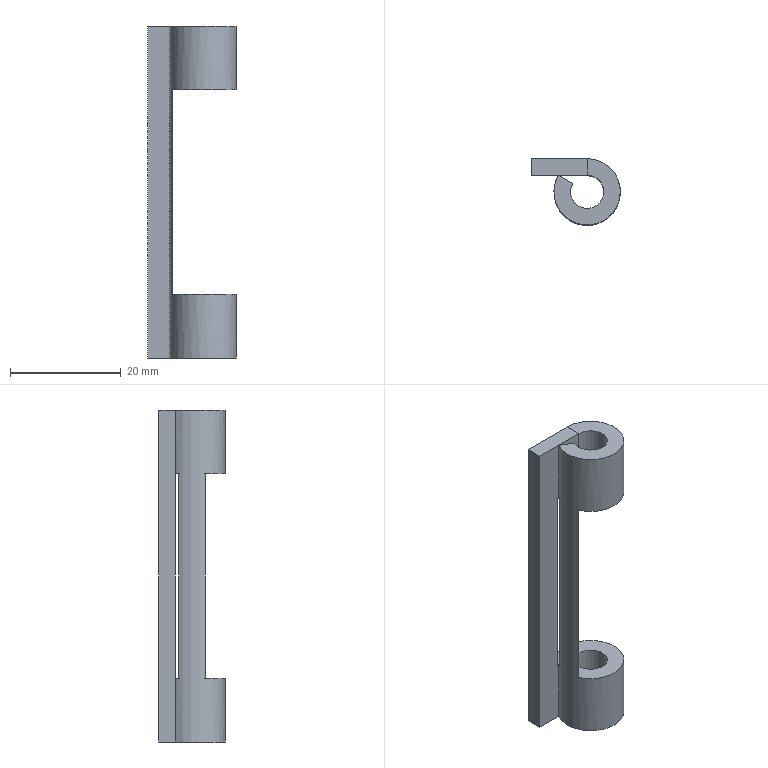Part | SolidWorks | features Cut 1, FlatPattern 1, Hem 1, SMBaseFlange 1, SheetMetal 1 | 1 solid | 16 faces | box 16 x 12 x 60 mm | volume 2875 mm3 | plane 13 | cylinder 3 | commonest cylinder face diameters 6 x2 12 x1
STEP:
#1=CARTESIAN_POINT('',(-3.5,-3.,-18.5));
#2=VERTEX_POINT('',#1);
#3=CARTESIAN_POINT('',(2.,-3.,-18.5));
#4=VERTEX_POINT('',#3);
#5=CARTESIAN_POINT('',(0.,-3.,-18.5));
#6=DIRECTION('',(1.,0.,0.));
#7=VECTOR('',#6,1000.);
#8=LINE('',#5,#7);
#9=EDGE_CURVE('',#2,#4,#8,.T.);
#10=ORIENTED_EDGE('',*,*,#9,.F.);
#11=CARTESIAN_POINT('',(-3.5,-3.,18.5));
#12=VERTEX_POINT('',#11);
#13=CARTESIAN_POINT('',(-3.5,-3.,0.));
#14=DIRECTION('',(0.,0.,1.));
#15=VECTOR('',#14,1000.);
#16=LINE('',#13,#15);
#17=EDGE_CURVE('',#2,#12,#16,.T.);
#18=ORIENTED_EDGE('',*,*,#17,.T.);
#19=CARTESIAN_POINT('',(2.,-3.,18.5));
#20=VERTEX_POINT('',#19);
#21=CARTESIAN_POINT('',(0.,-3.,18.5));
#22=DIRECTION('',(1.,0.,0.));
#23=VECTOR('',#22,1000.);
#24=LINE('',#21,#23);
#25=EDGE_CURVE('',#12,#20,#24,.T.);
#26=ORIENTED_EDGE('',*,*,#25,.T.);
#27=CARTESIAN_POINT('',(2.,-3.,30.));
#28=VERTEX_POINT('',#27);
#29=CARTESIAN_POINT('',(2.,-3.,30.));
#30=DIRECTION('',(0.,0.,-1.));
#31=VECTOR('',#30,1000.);
#32=LINE('',#29,#31);
#33=EDGE_CURVE('',#28,#20,#32,.T.);
#34=ORIENTED_EDGE('',*,*,#33,.F.);
#35=CARTESIAN_POINT('',(-8.,-3.,30.));
#36=VERTEX_POINT('',#35);
#37=CARTESIAN_POINT('',(-8.,-3.,30.));
#38=DIRECTION('',(1.,0.,0.));
#39=VECTOR('',#38,1000.);
#40=LINE('',#37,#39);
#41=EDGE_CURVE('',#36,#28,#40,.T.);
#42=ORIENTED_EDGE('',*,*,#41,.F.);
#43=CARTESIAN_POINT('',(-8.,-3.,-30.));
#44=VERTEX_POINT('',#43);
#45=CARTESIAN_POINT('',(-8.,-3.,-30.));
#46=DIRECTION('',(0.,0.,1.));
#47=VECTOR('',#46,1000.);
#48=LINE('',#45,#47);
#49=EDGE_CURVE('',#44,#36,#48,.T.);
#50=ORIENTED_EDGE('',*,*,#49,.F.);
#51=CARTESIAN_POINT('',(2.,-3.,-30.));
#52=VERTEX_POINT('',#51);
#53=CARTESIAN_POINT('',(-8.,-3.,-30.));
#54=DIRECTION('',(-1.,0.,0.));
#55=VECTOR('',#54,1000.);
#56=LINE('',#53,#55);
#57=EDGE_CURVE('',#52,#44,#56,.T.);
#58=ORIENTED_EDGE('',*,*,#57,.F.);
#59=CARTESIAN_POINT('',(2.,-3.,30.));
#60=DIRECTION('',(0.,0.,-1.));
#61=VECTOR('',#60,1000.);
#62=LINE('',#59,#61);
#63=EDGE_CURVE('',#4,#52,#62,.T.);
#64=ORIENTED_EDGE('',*,*,#63,.F.);
#65=EDGE_LOOP('',(#10,#18,#26,#34,#42,#50,#58,#64));
#66=FACE_OUTER_BOUND('',#65,.T.);
#67=CARTESIAN_POINT('',(0.,-3.,0.));
#68=DIRECTION('',(0.,1.,0.));
#69=DIRECTION('',(0.,0.,1.));
#70=AXIS2_PLACEMENT_3D('',#67,#68,#69);
#71=PLANE('',#70);
#72=ADVANCED_FACE('',(#66),#71,.F.);
#73=CARTESIAN_POINT('',(-3.5,0.,-18.5));
#74=VERTEX_POINT('',#73);
#75=CARTESIAN_POINT('',(-3.5,0.,18.5));
#76=VERTEX_POINT('',#75);
#77=CARTESIAN_POINT('',(-3.5,0.,-18.5));
#78=DIRECTION('',(0.,0.,1.));
#79=VECTOR('',#78,1000.);
#80=LINE('',#77,#79);
#81=EDGE_CURVE('',#74,#76,#80,.T.);
#82=ORIENTED_EDGE('',*,*,#81,.F.);
#83=CARTESIAN_POINT('',(2.,0.,-18.5));
#84=VERTEX_POINT('',#83);
#85=CARTESIAN_POINT('',(-3.5,0.,-18.5));
#86=DIRECTION('',(1.,0.,0.));
#87=VECTOR('',#86,1000.);
#88=LINE('',#85,#87);
#89=EDGE_CURVE('',#74,#84,#88,.T.);
#90=ORIENTED_EDGE('',*,*,#89,.T.);
#91=CARTESIAN_POINT('',(2.,0.,-30.));
#92=VERTEX_POINT('',#91);
#93=CARTESIAN_POINT('',(2.,0.,30.));
#94=DIRECTION('',(0.,0.,-1.));
#95=VECTOR('',#94,1000.);
#96=LINE('',#93,#95);
#97=EDGE_CURVE('',#84,#92,#96,.T.);
#98=ORIENTED_EDGE('',*,*,#97,.T.);
#99=CARTESIAN_POINT('',(-8.,0.,-30.));
#100=VERTEX_POINT('',#99);
#101=CARTESIAN_POINT('',(-8.,0.,-30.));
#102=DIRECTION('',(-1.,0.,0.));
#103=VECTOR('',#102,1000.);
#104=LINE('',#101,#103);
#105=EDGE_CURVE('',#92,#100,#104,.T.);
#106=ORIENTED_EDGE('',*,*,#105,.T.);
#107=CARTESIAN_POINT('',(-8.,0.,30.));
#108=VERTEX_POINT('',#107);
#109=CARTESIAN_POINT('',(-8.,0.,-30.));
#110=DIRECTION('',(0.,0.,1.));
#111=VECTOR('',#110,1000.);
#112=LINE('',#109,#111);
#113=EDGE_CURVE('',#100,#108,#112,.T.);
#114=ORIENTED_EDGE('',*,*,#113,.T.);
#115=CARTESIAN_POINT('',(2.,0.,30.));
#116=VERTEX_POINT('',#115);
#117=CARTESIAN_POINT('',(-8.,0.,30.));
#118=DIRECTION('',(1.,0.,0.));
#119=VECTOR('',#118,1000.);
#120=LINE('',#117,#119);
#121=EDGE_CURVE('',#108,#116,#120,.T.);
#122=ORIENTED_EDGE('',*,*,#121,.T.);
#123=CARTESIAN_POINT('',(2.,0.,18.5));
#124=VERTEX_POINT('',#123);
#125=CARTESIAN_POINT('',(2.,0.,30.));
#126=DIRECTION('',(0.,0.,-1.));
#127=VECTOR('',#126,1000.);
#128=LINE('',#125,#127);
#129=EDGE_CURVE('',#116,#124,#128,.T.);
#130=ORIENTED_EDGE('',*,*,#129,.T.);
#131=CARTESIAN_POINT('',(-3.5,0.,18.5));
#132=DIRECTION('',(1.,0.,0.));
#133=VECTOR('',#132,1000.);
#134=LINE('',#131,#133);
#135=EDGE_CURVE('',#76,#124,#134,.T.);
#136=ORIENTED_EDGE('',*,*,#135,.F.);
#137=EDGE_LOOP('',(#82,#90,#98,#106,#114,#122,#130,#136));
#138=FACE_OUTER_BOUND('',#137,.T.);
#139=CARTESIAN_POINT('',(0.,0.,0.));
#140=DIRECTION('',(0.,1.,0.));
#141=DIRECTION('',(0.,0.,1.));
#142=AXIS2_PLACEMENT_3D('',#139,#140,#141);
#143=PLANE('',#142);
#144=ADVANCED_FACE('',(#138),#143,.T.);
#145=CARTESIAN_POINT('',(-3.196,-3.,-30.));
#146=VERTEX_POINT('',#145);
#147=CARTESIAN_POINT('',(-3.196,-3.,-18.5));
#148=VERTEX_POINT('',#147);
#149=CARTESIAN_POINT('',(-3.196,-3.,30.));
#150=DIRECTION('',(0.,0.,1.));
#151=VECTOR('',#150,1000.);
#152=LINE('',#149,#151);
#153=EDGE_CURVE('',#146,#148,#152,.T.);
#154=ORIENTED_EDGE('',*,*,#153,.T.);
#155=CARTESIAN_POINT('',(-0.5981,-4.5,-18.5));
#156=VERTEX_POINT('',#155);
#157=CARTESIAN_POINT('',(-0.5981,-4.5,-18.5));
#158=DIRECTION('',(0.866,-0.5,0.));
#159=VECTOR('',#158,1000.);
#160=LINE('',#157,#159);
#161=EDGE_CURVE('',#148,#156,#160,.T.);
#162=ORIENTED_EDGE('',*,*,#161,.T.);
#163=CARTESIAN_POINT('',(-0.5981,-4.5,-30.));
#164=VERTEX_POINT('',#163);
#165=CARTESIAN_POINT('',(-0.5981,-4.5,30.));
#166=DIRECTION('',(0.,0.,1.));
#167=VECTOR('',#166,1000.);
#168=LINE('',#165,#167);
#169=EDGE_CURVE('',#164,#156,#168,.T.);
#170=ORIENTED_EDGE('',*,*,#169,.F.);
#171=CARTESIAN_POINT('',(-0.5981,-4.5,-30.));
#172=DIRECTION('',(-0.866,0.5,0.));
#173=VECTOR('',#172,1000.);
#174=LINE('',#171,#173);
#175=EDGE_CURVE('',#164,#146,#174,.T.);
#176=ORIENTED_EDGE('',*,*,#175,.T.);
#177=EDGE_LOOP('',(#154,#162,#170,#176));
#178=FACE_OUTER_BOUND('',#177,.T.);
#179=CARTESIAN_POINT('',(-0.5981,-4.5,0.));
#180=DIRECTION('',(-0.5,-0.866,0.));
#181=DIRECTION('',(0.,0.,1.));
#182=AXIS2_PLACEMENT_3D('',#179,#180,#181);
#183=PLANE('',#182);
#184=ADVANCED_FACE('',(#178),#183,.F.);
#185=ORIENTED_EDGE('',*,*,#97,.F.);
#186=CARTESIAN_POINT('',(-3.5,-8.398,-18.5));
#187=VERTEX_POINT('',#186);
#188=CARTESIAN_POINT('',(2.,-6.,-18.5));
#189=DIRECTION('',(0.,0.,-1.));
#190=DIRECTION('',(1.,0.,0.));
#191=AXIS2_PLACEMENT_3D('',#188,#189,#190);
#192=CIRCLE('',#191,6.);
#193=EDGE_CURVE('',#84,#187,#192,.T.);
#194=ORIENTED_EDGE('',*,*,#193,.T.);
#195=CARTESIAN_POINT('',(-3.5,-8.398,18.5));
#196=VERTEX_POINT('',#195);
#197=CARTESIAN_POINT('',(-3.5,-8.398,30.));
#198=DIRECTION('',(0.,0.,-1.));
#199=VECTOR('',#198,1000.);
#200=LINE('',#197,#199);
#201=EDGE_CURVE('',#196,#187,#200,.T.);
#202=ORIENTED_EDGE('',*,*,#201,.F.);
#203=CARTESIAN_POINT('',(2.,-6.,18.5));
#204=DIRECTION('',(0.,0.,-1.));
#205=DIRECTION('',(1.,0.,0.));
#206=AXIS2_PLACEMENT_3D('',#203,#204,#205);
#207=CIRCLE('',#206,6.);
#208=EDGE_CURVE('',#124,#196,#207,.T.);
#209=ORIENTED_EDGE('',*,*,#208,.F.);
#210=ORIENTED_EDGE('',*,*,#129,.F.);
#211=CARTESIAN_POINT('',(-3.196,-3.,30.));
#212=VERTEX_POINT('',#211);
#213=CARTESIAN_POINT('',(2.,-6.,30.));
#214=DIRECTION('',(0.,0.,1.));
#215=DIRECTION('',(1.,0.,0.));
#216=AXIS2_PLACEMENT_3D('',#213,#214,#215);
#217=CIRCLE('',#216,6.);
#218=EDGE_CURVE('',#212,#116,#217,.T.);
#219=ORIENTED_EDGE('',*,*,#218,.F.);
#220=CARTESIAN_POINT('',(-3.196,-3.,18.5));
#221=VERTEX_POINT('',#220);
#222=CARTESIAN_POINT('',(-3.196,-3.,30.));
#223=DIRECTION('',(0.,0.,1.));
#224=VECTOR('',#223,1000.);
#225=LINE('',#222,#224);
#226=EDGE_CURVE('',#221,#212,#225,.T.);
#227=ORIENTED_EDGE('',*,*,#226,.F.);
#228=CARTESIAN_POINT('',(-3.5,-3.602,18.5));
#229=VERTEX_POINT('',#228);
#230=CARTESIAN_POINT('',(2.,-6.,18.5));
#231=DIRECTION('',(0.,0.,-1.));
#232=DIRECTION('',(1.,0.,0.));
#233=AXIS2_PLACEMENT_3D('',#230,#231,#232);
#234=CIRCLE('',#233,6.);
#235=EDGE_CURVE('',#229,#221,#234,.T.);
#236=ORIENTED_EDGE('',*,*,#235,.F.);
#237=CARTESIAN_POINT('',(-3.5,-3.602,-18.5));
#238=VERTEX_POINT('',#237);
#239=CARTESIAN_POINT('',(-3.5,-3.602,30.));
#240=DIRECTION('',(0.,0.,1.));
#241=VECTOR('',#240,1000.);
#242=LINE('',#239,#241);
#243=EDGE_CURVE('',#238,#229,#242,.T.);
#244=ORIENTED_EDGE('',*,*,#243,.F.);
#245=CARTESIAN_POINT('',(2.,-6.,-18.5));
#246=DIRECTION('',(0.,0.,-1.));
#247=DIRECTION('',(1.,0.,0.));
#248=AXIS2_PLACEMENT_3D('',#245,#246,#247);
#249=CIRCLE('',#248,6.);
#250=EDGE_CURVE('',#238,#148,#249,.T.);
#251=ORIENTED_EDGE('',*,*,#250,.T.);
#252=ORIENTED_EDGE('',*,*,#153,.F.);
#253=CARTESIAN_POINT('',(2.,-6.,-30.));
#254=DIRECTION('',(0.,0.,-1.));
#255=DIRECTION('',(1.,0.,0.));
#256=AXIS2_PLACEMENT_3D('',#253,#254,#255);
#257=CIRCLE('',#256,6.);
#258=EDGE_CURVE('',#92,#146,#257,.T.);
#259=ORIENTED_EDGE('',*,*,#258,.F.);
#260=EDGE_LOOP('',(#185,#194,#202,#209,#210,#219,#227,#236,#244,#251,#252,#259));
#261=FACE_OUTER_BOUND('',#260,.T.);
#262=CARTESIAN_POINT('',(2.,-6.,30.));
#263=DIRECTION('',(0.,0.,1.));
#264=DIRECTION('',(-0.866,0.5,0.));
#265=AXIS2_PLACEMENT_3D('',#262,#263,#264);
#266=CYLINDRICAL_SURFACE('',#265,6.);
#267=ADVANCED_FACE('',(#261),#266,.T.);
#268=CARTESIAN_POINT('',(2.,-6.,-18.5));
#269=DIRECTION('',(0.,0.,-1.));
#270=DIRECTION('',(1.,0.,0.));
#271=AXIS2_PLACEMENT_3D('',#268,#269,#270);
#272=CIRCLE('',#271,3.);
#273=EDGE_CURVE('',#4,#156,#272,.T.);
#274=ORIENTED_EDGE('',*,*,#273,.F.);
#275=ORIENTED_EDGE('',*,*,#63,.T.);
#276=CARTESIAN_POINT('',(2.,-6.,-30.));
#277=DIRECTION('',(0.,0.,-1.));
#278=DIRECTION('',(1.,0.,0.));
#279=AXIS2_PLACEMENT_3D('',#276,#277,#278);
#280=CIRCLE('',#279,3.);
#281=EDGE_CURVE('',#52,#164,#280,.T.);
#282=ORIENTED_EDGE('',*,*,#281,.T.);
#283=ORIENTED_EDGE('',*,*,#169,.T.);
#284=EDGE_LOOP('',(#274,#275,#282,#283));
#285=FACE_OUTER_BOUND('',#284,.T.);
#286=CARTESIAN_POINT('',(2.,-6.,30.));
#287=DIRECTION('',(0.,0.,1.));
#288=DIRECTION('',(-0.866,0.5,0.));
#289=AXIS2_PLACEMENT_3D('',#286,#287,#288);
#290=CYLINDRICAL_SURFACE('',#289,3.);
#291=ADVANCED_FACE('',(#285),#290,.F.);
#292=ORIENTED_EDGE('',*,*,#41,.T.);
#293=CARTESIAN_POINT('',(2.,-3.,30.));
#294=DIRECTION('',(0.,1.,0.));
#295=VECTOR('',#294,1000.);
#296=LINE('',#293,#295);
#297=EDGE_CURVE('',#28,#116,#296,.T.);
#298=ORIENTED_EDGE('',*,*,#297,.T.);
#299=ORIENTED_EDGE('',*,*,#121,.F.);
#300=CARTESIAN_POINT('',(-8.,-3.,30.));
#301=DIRECTION('',(0.,1.,0.));
#302=VECTOR('',#301,1000.);
#303=LINE('',#300,#302);
#304=EDGE_CURVE('',#36,#108,#303,.T.);
#305=ORIENTED_EDGE('',*,*,#304,.F.);
#306=EDGE_LOOP('',(#292,#298,#299,#305));
#307=FACE_OUTER_BOUND('',#306,.T.);
#308=CARTESIAN_POINT('',(-8.,-3.,30.));
#309=DIRECTION('',(0.,0.,1.));
#310=DIRECTION('',(1.,0.,0.));
#311=AXIS2_PLACEMENT_3D('',#308,#309,#310);
#312=PLANE('',#311);
#313=ADVANCED_FACE('',(#307),#312,.T.);
#314=ORIENTED_EDGE('',*,*,#113,.F.);
#315=CARTESIAN_POINT('',(-8.,-3.,-30.));
#316=DIRECTION('',(0.,1.,0.));
#317=VECTOR('',#316,1000.);
#318=LINE('',#315,#317);
#319=EDGE_CURVE('',#44,#100,#318,.T.);
#320=ORIENTED_EDGE('',*,*,#319,.F.);
#321=ORIENTED_EDGE('',*,*,#49,.T.);
#322=ORIENTED_EDGE('',*,*,#304,.T.);
#323=EDGE_LOOP('',(#314,#320,#321,#322));
#324=FACE_OUTER_BOUND('',#323,.T.);
#325=CARTESIAN_POINT('',(-8.,-3.,-30.));
#326=DIRECTION('',(-1.,0.,0.));
#327=DIRECTION('',(0.,0.,1.));
#328=AXIS2_PLACEMENT_3D('',#325,#326,#327);
#329=PLANE('',#328);
#330=ADVANCED_FACE('',(#324),#329,.T.);
#331=CARTESIAN_POINT('',(2.,-3.,-30.));
#332=DIRECTION('',(0.,1.,0.));
#333=VECTOR('',#332,1000.);
#334=LINE('',#331,#333);
#335=EDGE_CURVE('',#52,#92,#334,.T.);
#336=ORIENTED_EDGE('',*,*,#335,.F.);
#337=ORIENTED_EDGE('',*,*,#57,.T.);
#338=ORIENTED_EDGE('',*,*,#319,.T.);
#339=ORIENTED_EDGE('',*,*,#105,.F.);
#340=EDGE_LOOP('',(#336,#337,#338,#339));
#341=FACE_OUTER_BOUND('',#340,.T.);
#342=CARTESIAN_POINT('',(-8.,-3.,-30.));
#343=DIRECTION('',(0.,0.,-1.));
#344=DIRECTION('',(-1.,0.,0.));
#345=AXIS2_PLACEMENT_3D('',#342,#343,#344);
#346=PLANE('',#345);
#347=ADVANCED_FACE('',(#341),#346,.T.);
#348=CARTESIAN_POINT('',(-0.5981,-4.5,18.5));
#349=VERTEX_POINT('',#348);
#350=CARTESIAN_POINT('',(-0.5981,-4.5,18.5));
#351=DIRECTION('',(0.866,-0.5,0.));
#352=VECTOR('',#351,1000.);
#353=LINE('',#350,#352);
#354=EDGE_CURVE('',#221,#349,#353,.T.);
#355=ORIENTED_EDGE('',*,*,#354,.F.);
#356=ORIENTED_EDGE('',*,*,#226,.T.);
#357=CARTESIAN_POINT('',(-0.5981,-4.5,30.));
#358=VERTEX_POINT('',#357);
#359=CARTESIAN_POINT('',(-0.5981,-4.5,30.));
#360=DIRECTION('',(-0.866,0.5,0.));
#361=VECTOR('',#360,1000.);
#362=LINE('',#359,#361);
#363=EDGE_CURVE('',#358,#212,#362,.T.);
#364=ORIENTED_EDGE('',*,*,#363,.F.);
#365=CARTESIAN_POINT('',(-0.5981,-4.5,30.));
#366=DIRECTION('',(0.,0.,1.));
#367=VECTOR('',#366,1000.);
#368=LINE('',#365,#367);
#369=EDGE_CURVE('',#349,#358,#368,.T.);
#370=ORIENTED_EDGE('',*,*,#369,.F.);
#371=EDGE_LOOP('',(#355,#356,#364,#370));
#372=FACE_OUTER_BOUND('',#371,.T.);
#373=CARTESIAN_POINT('',(-0.5981,-4.5,0.));
#374=DIRECTION('',(-0.5,-0.866,0.));
#375=DIRECTION('',(0.,0.,1.));
#376=AXIS2_PLACEMENT_3D('',#373,#374,#375);
#377=PLANE('',#376);
#378=ADVANCED_FACE('',(#372),#377,.F.);
#379=ORIENTED_EDGE('',*,*,#175,.F.);
#380=ORIENTED_EDGE('',*,*,#281,.F.);
#381=ORIENTED_EDGE('',*,*,#335,.T.);
#382=ORIENTED_EDGE('',*,*,#258,.T.);
#383=EDGE_LOOP('',(#379,#380,#381,#382));
#384=FACE_OUTER_BOUND('',#383,.T.);
#385=CARTESIAN_POINT('',(2.,-6.,-30.));
#386=DIRECTION('',(0.,0.,-1.));
#387=DIRECTION('',(-1.,0.,0.));
#388=AXIS2_PLACEMENT_3D('',#385,#386,#387);
#389=PLANE('',#388);
#390=ADVANCED_FACE('',(#384),#389,.T.);
#391=CARTESIAN_POINT('',(2.,-6.,30.));
#392=DIRECTION('',(0.,0.,1.));
#393=DIRECTION('',(1.,0.,0.));
#394=AXIS2_PLACEMENT_3D('',#391,#392,#393);
#395=CIRCLE('',#394,3.);
#396=EDGE_CURVE('',#358,#28,#395,.T.);
#397=ORIENTED_EDGE('',*,*,#396,.F.);
#398=ORIENTED_EDGE('',*,*,#363,.T.);
#399=ORIENTED_EDGE('',*,*,#218,.T.);
#400=ORIENTED_EDGE('',*,*,#297,.F.);
#401=EDGE_LOOP('',(#397,#398,#399,#400));
#402=FACE_OUTER_BOUND('',#401,.T.);
#403=CARTESIAN_POINT('',(2.,-6.,30.));
#404=DIRECTION('',(0.,0.,-1.));
#405=DIRECTION('',(-1.,0.,0.));
#406=AXIS2_PLACEMENT_3D('',#403,#404,#405);
#407=PLANE('',#406);
#408=ADVANCED_FACE('',(#402),#407,.F.);
#409=ORIENTED_EDGE('',*,*,#33,.T.);
#410=CARTESIAN_POINT('',(2.,-6.,18.5));
#411=DIRECTION('',(0.,0.,-1.));
#412=DIRECTION('',(1.,0.,0.));
#413=AXIS2_PLACEMENT_3D('',#410,#411,#412);
#414=CIRCLE('',#413,3.);
#415=EDGE_CURVE('',#20,#349,#414,.T.);
#416=ORIENTED_EDGE('',*,*,#415,.T.);
#417=ORIENTED_EDGE('',*,*,#369,.T.);
#418=ORIENTED_EDGE('',*,*,#396,.T.);
#419=EDGE_LOOP('',(#409,#416,#417,#418));
#420=FACE_OUTER_BOUND('',#419,.T.);
#421=CARTESIAN_POINT('',(2.,-6.,30.));
#422=DIRECTION('',(0.,0.,1.));
#423=DIRECTION('',(-0.866,0.5,0.));
#424=AXIS2_PLACEMENT_3D('',#421,#422,#423);
#425=CYLINDRICAL_SURFACE('',#424,3.);
#426=ADVANCED_FACE('',(#420),#425,.F.);
#427=CARTESIAN_POINT('',(-3.5,-15.,-18.5));
#428=DIRECTION('',(0.,1.,0.));
#429=VECTOR('',#428,1000.);
#430=LINE('',#427,#429);
#431=EDGE_CURVE('',#2,#74,#430,.T.);
#432=ORIENTED_EDGE('',*,*,#431,.T.);
#433=ORIENTED_EDGE('',*,*,#81,.T.);
#434=CARTESIAN_POINT('',(-3.5,-15.,18.5));
#435=DIRECTION('',(0.,1.,0.));
#436=VECTOR('',#435,1000.);
#437=LINE('',#434,#436);
#438=EDGE_CURVE('',#12,#76,#437,.T.);
#439=ORIENTED_EDGE('',*,*,#438,.F.);
#440=ORIENTED_EDGE('',*,*,#17,.F.);
#441=EDGE_LOOP('',(#432,#433,#439,#440));
#442=FACE_OUTER_BOUND('',#441,.T.);
#443=CARTESIAN_POINT('',(-3.5,-15.,-18.5));
#444=DIRECTION('',(-1.,0.,0.));
#445=DIRECTION('',(0.,0.,1.));
#446=AXIS2_PLACEMENT_3D('',#443,#444,#445);
#447=PLANE('',#446);
#448=ADVANCED_FACE('',(#442),#447,.F.);
#449=ORIENTED_EDGE('',*,*,#201,.T.);
#450=CARTESIAN_POINT('',(-3.5,-15.,-18.5));
#451=DIRECTION('',(0.,1.,0.));
#452=VECTOR('',#451,1000.);
#453=LINE('',#450,#452);
#454=EDGE_CURVE('',#187,#238,#453,.T.);
#455=ORIENTED_EDGE('',*,*,#454,.T.);
#456=ORIENTED_EDGE('',*,*,#243,.T.);
#457=CARTESIAN_POINT('',(-3.5,-15.,18.5));
#458=DIRECTION('',(0.,1.,0.));
#459=VECTOR('',#458,1000.);
#460=LINE('',#457,#459);
#461=EDGE_CURVE('',#196,#229,#460,.T.);
#462=ORIENTED_EDGE('',*,*,#461,.F.);
#463=EDGE_LOOP('',(#449,#455,#456,#462));
#464=FACE_OUTER_BOUND('',#463,.T.);
#465=CARTESIAN_POINT('',(-3.5,-15.,-18.5));
#466=DIRECTION('',(-1.,0.,0.));
#467=DIRECTION('',(0.,0.,1.));
#468=AXIS2_PLACEMENT_3D('',#465,#466,#467);
#469=PLANE('',#468);
#470=ADVANCED_FACE('',(#464),#469,.F.);
#471=ORIENTED_EDGE('',*,*,#193,.F.);
#472=ORIENTED_EDGE('',*,*,#89,.F.);
#473=ORIENTED_EDGE('',*,*,#431,.F.);
#474=ORIENTED_EDGE('',*,*,#9,.T.);
#475=ORIENTED_EDGE('',*,*,#273,.T.);
#476=ORIENTED_EDGE('',*,*,#161,.F.);
#477=ORIENTED_EDGE('',*,*,#250,.F.);
#478=ORIENTED_EDGE('',*,*,#454,.F.);
#479=EDGE_LOOP('',(#471,#472,#473,#474,#475,#476,#477,#478));
#480=FACE_OUTER_BOUND('',#479,.T.);
#481=CARTESIAN_POINT('',(-3.5,-15.,-18.5));
#482=DIRECTION('',(0.,0.,1.));
#483=DIRECTION('',(1.,0.,0.));
#484=AXIS2_PLACEMENT_3D('',#481,#482,#483);
#485=PLANE('',#484);
#486=ADVANCED_FACE('',(#480),#485,.T.);
#487=ORIENTED_EDGE('',*,*,#208,.T.);
#488=ORIENTED_EDGE('',*,*,#461,.T.);
#489=ORIENTED_EDGE('',*,*,#235,.T.);
#490=ORIENTED_EDGE('',*,*,#354,.T.);
#491=ORIENTED_EDGE('',*,*,#415,.F.);
#492=ORIENTED_EDGE('',*,*,#25,.F.);
#493=ORIENTED_EDGE('',*,*,#438,.T.);
#494=ORIENTED_EDGE('',*,*,#135,.T.);
#495=EDGE_LOOP('',(#487,#488,#489,#490,#491,#492,#493,#494));
#496=FACE_OUTER_BOUND('',#495,.T.);
#497=CARTESIAN_POINT('',(-3.5,-15.,18.5));
#498=DIRECTION('',(0.,0.,1.));
#499=DIRECTION('',(1.,0.,0.));
#500=AXIS2_PLACEMENT_3D('',#497,#498,#499);
#501=PLANE('',#500);
#502=ADVANCED_FACE('',(#496),#501,.F.);
#503=CLOSED_SHELL('',(#72,#144,#184,#267,#291,#313,#330,#347,#378,#390,#408,#426,#448,#470,#486,#502));
#504=MANIFOLD_SOLID_BREP('',#503);
#505=CARTESIAN_POINT('',(0.,0.,0.));
#506=DIRECTION('',(0.,0.,1.));
#507=DIRECTION('',(1.,0.,0.));
#508=AXIS2_PLACEMENT_3D('',#505,#506,#507);
#509=(LENGTH_UNIT()NAMED_UNIT(*)SI_UNIT(.MILLI.,.METRE.));
#510=UNCERTAINTY_MEASURE_WITH_UNIT(LENGTH_MEASURE(0.00001),#509,'','');
#511=(NAMED_UNIT(*)PLANE_ANGLE_UNIT()SI_UNIT($,.RADIAN.));
#512=(NAMED_UNIT(*)SI_UNIT($,.STERADIAN.)SOLID_ANGLE_UNIT());
#513=(GEOMETRIC_REPRESENTATION_CONTEXT(3)GLOBAL_UNCERTAINTY_ASSIGNED_CONTEXT((#510))GLOBAL_UNIT_ASSIGNED_CONTEXT((#509,#511,#512))REPRESENTATION_CONTEXT('',''));
#514=ADVANCED_BREP_SHAPE_REPRESENTATION('',(#504,#508),#513);